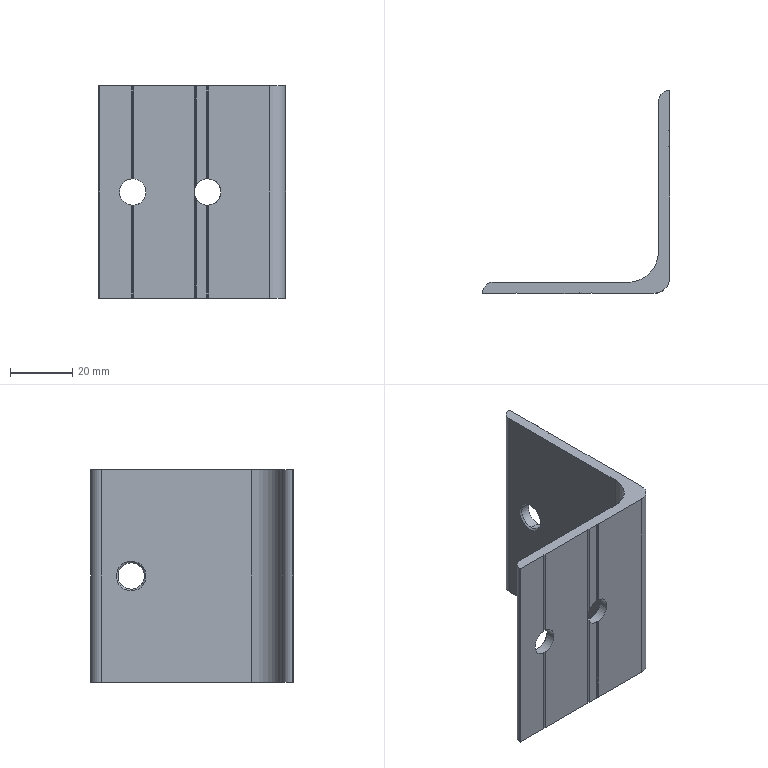Part | STEP file | 31E-01022QY13 | 1 solid | 65 faces | box 60 x 64.996 x 68 mm | volume 29020 mm3 | cylinder 30 | plane 29 | cone 6 | commonest cylinder face diameters 0.2 x17 8.5 x6 0.4 x3 7 x2 10 x1 20 x1